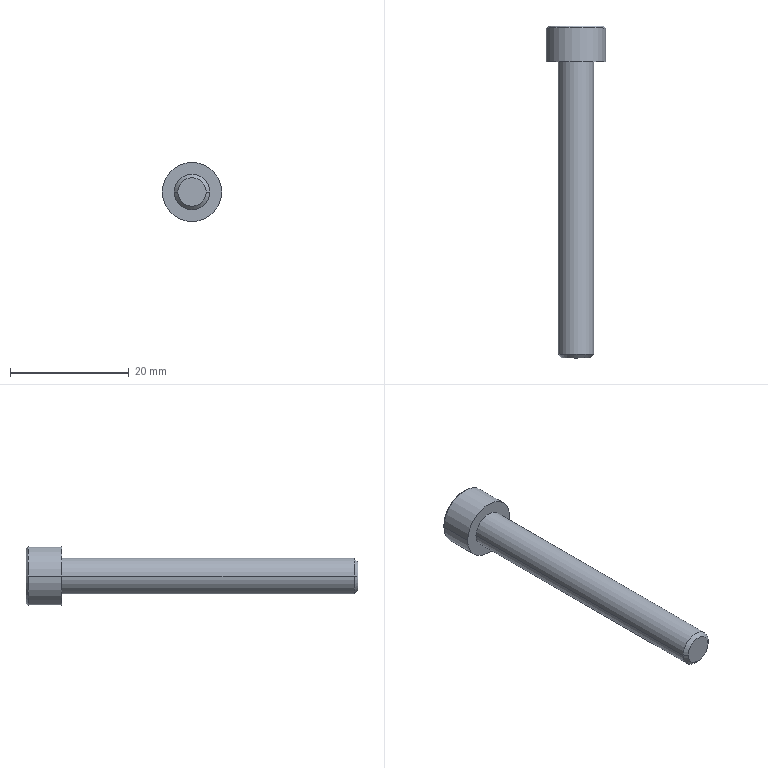Part | SolidWorks | features BaseBody 1, MoveFace 1 | 1 solid | 18 faces | box 10 x 56 x 10 mm | volume 1814 mm3 | plane 10 | cylinder 4 | cone 4 | commonest cylinder face diameters 6 x2 10 x2
STEP:
#1=CARTESIAN_POINT('',(-5.,8.,0.));
#2=VERTEX_POINT('',#1);
#3=CARTESIAN_POINT('',(5.,8.,0.));
#4=VERTEX_POINT('',#3);
#5=CARTESIAN_POINT('',(0.,8.,0.));
#6=DIRECTION('',(0.,1.,0.));
#7=DIRECTION('',(-1.,0.,0.));
#8=AXIS2_PLACEMENT_3D('',#5,#6,#7);
#9=CIRCLE('',#8,5.);
#10=EDGE_CURVE('',#2,#4,#9,.T.);
#11=ORIENTED_EDGE('',*,*,#10,.T.);
#12=CARTESIAN_POINT('',(5.,13.667,0.));
#13=VERTEX_POINT('',#12);
#14=CARTESIAN_POINT('',(5.,0.,0.));
#15=DIRECTION('',(0.,1.,0.));
#16=VECTOR('',#15,1000.);
#17=LINE('',#14,#16);
#18=EDGE_CURVE('',#4,#13,#17,.T.);
#19=ORIENTED_EDGE('',*,*,#18,.T.);
#20=CARTESIAN_POINT('',(-5.,13.667,0.));
#21=VERTEX_POINT('',#20);
#22=CARTESIAN_POINT('',(0.,13.667,0.));
#23=DIRECTION('',(0.,-1.,0.));
#24=DIRECTION('',(-1.,0.,0.));
#25=AXIS2_PLACEMENT_3D('',#22,#23,#24);
#26=CIRCLE('',#25,5.);
#27=EDGE_CURVE('',#13,#21,#26,.T.);
#28=ORIENTED_EDGE('',*,*,#27,.T.);
#29=CARTESIAN_POINT('',(-5.,0.,0.));
#30=DIRECTION('',(0.,1.,0.));
#31=VECTOR('',#30,1000.);
#32=LINE('',#29,#31);
#33=EDGE_CURVE('',#2,#21,#32,.T.);
#34=ORIENTED_EDGE('',*,*,#33,.F.);
#35=EDGE_LOOP('',(#11,#19,#28,#34));
#36=FACE_OUTER_BOUND('',#35,.T.);
#37=CARTESIAN_POINT('',(0.,0.,0.));
#38=DIRECTION('',(0.,1.,0.));
#39=DIRECTION('',(-1.,0.,0.));
#40=AXIS2_PLACEMENT_3D('',#37,#38,#39);
#41=CYLINDRICAL_SURFACE('',#40,5.);
#42=ADVANCED_FACE('',(#36),#41,.T.);
#43=CARTESIAN_POINT('',(4.667,14.,0.));
#44=VERTEX_POINT('',#43);
#45=CARTESIAN_POINT('',(-4.667,14.,0.));
#46=VERTEX_POINT('',#45);
#47=CARTESIAN_POINT('',(0.,14.,0.));
#48=DIRECTION('',(0.,-1.,0.));
#49=DIRECTION('',(1.,0.,0.));
#50=AXIS2_PLACEMENT_3D('',#47,#48,#49);
#51=CIRCLE('',#50,4.667);
#52=EDGE_CURVE('',#44,#46,#51,.T.);
#53=ORIENTED_EDGE('',*,*,#52,.T.);
#54=CARTESIAN_POINT('',(-5.,13.667,0.));
#55=DIRECTION('',(-0.7071,-0.7071,0.));
#56=VECTOR('',#55,1000.);
#57=LINE('',#54,#56);
#58=EDGE_CURVE('',#46,#21,#57,.T.);
#59=ORIENTED_EDGE('',*,*,#58,.T.);
#60=ORIENTED_EDGE('',*,*,#27,.F.);
#61=CARTESIAN_POINT('',(5.,13.667,0.));
#62=DIRECTION('',(0.7071,-0.7071,0.));
#63=VECTOR('',#62,1000.);
#64=LINE('',#61,#63);
#65=EDGE_CURVE('',#44,#13,#64,.T.);
#66=ORIENTED_EDGE('',*,*,#65,.F.);
#67=EDGE_LOOP('',(#53,#59,#60,#66));
#68=FACE_OUTER_BOUND('',#67,.T.);
#69=CARTESIAN_POINT('',(0.,13.667,0.));
#70=DIRECTION('',(0.,-1.,0.));
#71=DIRECTION('',(1.,0.,0.));
#72=AXIS2_PLACEMENT_3D('',#69,#70,#71);
#73=CONICAL_SURFACE('',#72,5.,0.7854);
#74=ADVANCED_FACE('',(#68),#73,.T.);
#75=CARTESIAN_POINT('',(-3.,-41.386,0.));
#76=VERTEX_POINT('',#75);
#77=CARTESIAN_POINT('',(3.,-41.386,0.));
#78=VERTEX_POINT('',#77);
#79=CARTESIAN_POINT('',(0.,-41.386,0.));
#80=DIRECTION('',(0.,1.,0.));
#81=DIRECTION('',(-1.,0.,0.));
#82=AXIS2_PLACEMENT_3D('',#79,#80,#81);
#83=CIRCLE('',#82,3.);
#84=EDGE_CURVE('',#76,#78,#83,.T.);
#85=ORIENTED_EDGE('',*,*,#84,.T.);
#86=CARTESIAN_POINT('',(3.,8.,0.));
#87=VERTEX_POINT('',#86);
#88=CARTESIAN_POINT('',(3.,0.,0.));
#89=DIRECTION('',(0.,1.,0.));
#90=VECTOR('',#89,1000.);
#91=LINE('',#88,#90);
#92=EDGE_CURVE('',#78,#87,#91,.T.);
#93=ORIENTED_EDGE('',*,*,#92,.T.);
#94=CARTESIAN_POINT('',(-3.,8.,0.));
#95=VERTEX_POINT('',#94);
#96=CARTESIAN_POINT('',(0.,8.,0.));
#97=DIRECTION('',(0.,-1.,0.));
#98=DIRECTION('',(-1.,0.,0.));
#99=AXIS2_PLACEMENT_3D('',#96,#97,#98);
#100=CIRCLE('',#99,3.);
#101=EDGE_CURVE('',#87,#95,#100,.T.);
#102=ORIENTED_EDGE('',*,*,#101,.T.);
#103=CARTESIAN_POINT('',(-3.,0.,0.));
#104=DIRECTION('',(0.,1.,0.));
#105=VECTOR('',#104,1000.);
#106=LINE('',#103,#105);
#107=EDGE_CURVE('',#76,#95,#106,.T.);
#108=ORIENTED_EDGE('',*,*,#107,.F.);
#109=EDGE_LOOP('',(#85,#93,#102,#108));
#110=FACE_OUTER_BOUND('',#109,.T.);
#111=CARTESIAN_POINT('',(0.,0.,0.));
#112=DIRECTION('',(0.,1.,0.));
#113=DIRECTION('',(-1.,0.,0.));
#114=AXIS2_PLACEMENT_3D('',#111,#112,#113);
#115=CYLINDRICAL_SURFACE('',#114,3.);
#116=ADVANCED_FACE('',(#110),#115,.T.);
#117=CARTESIAN_POINT('',(-2.386,-42.,0.));
#118=VERTEX_POINT('',#117);
#119=CARTESIAN_POINT('',(2.386,-42.,0.));
#120=VERTEX_POINT('',#119);
#121=CARTESIAN_POINT('',(0.,-42.,0.));
#122=DIRECTION('',(0.,1.,0.));
#123=DIRECTION('',(-1.,0.,0.));
#124=AXIS2_PLACEMENT_3D('',#121,#122,#123);
#125=CIRCLE('',#124,2.386);
#126=EDGE_CURVE('',#118,#120,#125,.T.);
#127=ORIENTED_EDGE('',*,*,#126,.T.);
#128=CARTESIAN_POINT('',(3.,-41.386,0.));
#129=DIRECTION('',(0.7071,0.7071,0.));
#130=VECTOR('',#129,1000.);
#131=LINE('',#128,#130);
#132=EDGE_CURVE('',#120,#78,#131,.T.);
#133=ORIENTED_EDGE('',*,*,#132,.T.);
#134=ORIENTED_EDGE('',*,*,#84,.F.);
#135=CARTESIAN_POINT('',(-3.,-41.386,0.));
#136=DIRECTION('',(-0.7071,0.7071,0.));
#137=VECTOR('',#136,1000.);
#138=LINE('',#135,#137);
#139=EDGE_CURVE('',#118,#76,#138,.T.);
#140=ORIENTED_EDGE('',*,*,#139,.F.);
#141=EDGE_LOOP('',(#127,#133,#134,#140));
#142=FACE_OUTER_BOUND('',#141,.T.);
#143=CARTESIAN_POINT('',(0.,-41.386,0.));
#144=DIRECTION('',(0.,1.,0.));
#145=DIRECTION('',(-1.,0.,0.));
#146=AXIS2_PLACEMENT_3D('',#143,#144,#145);
#147=CONICAL_SURFACE('',#146,3.,0.7854);
#148=ADVANCED_FACE('',(#142),#147,.T.);
#149=ORIENTED_EDGE('',*,*,#18,.F.);
#150=CARTESIAN_POINT('',(0.,8.,0.));
#151=DIRECTION('',(0.,1.,0.));
#152=DIRECTION('',(-1.,0.,0.));
#153=AXIS2_PLACEMENT_3D('',#150,#151,#152);
#154=CIRCLE('',#153,5.);
#155=EDGE_CURVE('',#4,#2,#154,.T.);
#156=ORIENTED_EDGE('',*,*,#155,.T.);
#157=ORIENTED_EDGE('',*,*,#33,.T.);
#158=CARTESIAN_POINT('',(0.,13.667,0.));
#159=DIRECTION('',(0.,-1.,0.));
#160=DIRECTION('',(-1.,0.,0.));
#161=AXIS2_PLACEMENT_3D('',#158,#159,#160);
#162=CIRCLE('',#161,5.);
#163=EDGE_CURVE('',#21,#13,#162,.T.);
#164=ORIENTED_EDGE('',*,*,#163,.T.);
#165=EDGE_LOOP('',(#149,#156,#157,#164));
#166=FACE_OUTER_BOUND('',#165,.T.);
#167=CARTESIAN_POINT('',(0.,0.,0.));
#168=DIRECTION('',(0.,1.,0.));
#169=DIRECTION('',(-1.,0.,0.));
#170=AXIS2_PLACEMENT_3D('',#167,#168,#169);
#171=CYLINDRICAL_SURFACE('',#170,5.);
#172=ADVANCED_FACE('',(#166),#171,.T.);
#173=ORIENTED_EDGE('',*,*,#58,.F.);
#174=CARTESIAN_POINT('',(0.,14.,0.));
#175=DIRECTION('',(0.,-1.,0.));
#176=DIRECTION('',(1.,0.,0.));
#177=AXIS2_PLACEMENT_3D('',#174,#175,#176);
#178=CIRCLE('',#177,4.667);
#179=EDGE_CURVE('',#46,#44,#178,.T.);
#180=ORIENTED_EDGE('',*,*,#179,.T.);
#181=ORIENTED_EDGE('',*,*,#65,.T.);
#182=ORIENTED_EDGE('',*,*,#163,.F.);
#183=EDGE_LOOP('',(#173,#180,#181,#182));
#184=FACE_OUTER_BOUND('',#183,.T.);
#185=CARTESIAN_POINT('',(0.,13.667,0.));
#186=DIRECTION('',(0.,-1.,0.));
#187=DIRECTION('',(1.,0.,0.));
#188=AXIS2_PLACEMENT_3D('',#185,#186,#187);
#189=CONICAL_SURFACE('',#188,5.,0.7854);
#190=ADVANCED_FACE('',(#184),#189,.T.);
#191=ORIENTED_EDGE('',*,*,#10,.F.);
#192=ORIENTED_EDGE('',*,*,#155,.F.);
#193=EDGE_LOOP('',(#191,#192));
#194=FACE_OUTER_BOUND('',#193,.T.);
#195=CARTESIAN_POINT('',(0.,8.,0.));
#196=DIRECTION('',(0.,-1.,0.));
#197=DIRECTION('',(-1.,0.,0.));
#198=AXIS2_PLACEMENT_3D('',#195,#196,#197);
#199=CIRCLE('',#198,3.);
#200=EDGE_CURVE('',#95,#87,#199,.T.);
#201=ORIENTED_EDGE('',*,*,#200,.F.);
#202=ORIENTED_EDGE('',*,*,#101,.F.);
#203=EDGE_LOOP('',(#201,#202));
#204=FACE_BOUND('',#203,.T.);
#205=CARTESIAN_POINT('',(5.,8.,0.));
#206=DIRECTION('',(0.,1.,0.));
#207=DIRECTION('',(-1.,0.,0.));
#208=AXIS2_PLACEMENT_3D('',#205,#206,#207);
#209=PLANE('',#208);
#210=ADVANCED_FACE('',(#194,#204),#209,.F.);
#211=CARTESIAN_POINT('',(-2.51,14.,1.449));
#212=VERTEX_POINT('',#211);
#213=CARTESIAN_POINT('',(0.,14.,2.898));
#214=VERTEX_POINT('',#213);
#215=CARTESIAN_POINT('',(-2.51,14.,1.449));
#216=DIRECTION('',(0.866,0.,0.5));
#217=VECTOR('',#216,1000.);
#218=LINE('',#215,#217);
#219=EDGE_CURVE('',#212,#214,#218,.T.);
#220=ORIENTED_EDGE('',*,*,#219,.F.);
#221=CARTESIAN_POINT('',(-2.51,14.,-1.449));
#222=VERTEX_POINT('',#221);
#223=CARTESIAN_POINT('',(-2.51,14.,0.));
#224=DIRECTION('',(0.,0.,1.));
#225=VECTOR('',#224,1000.);
#226=LINE('',#223,#225);
#227=EDGE_CURVE('',#222,#212,#226,.T.);
#228=ORIENTED_EDGE('',*,*,#227,.F.);
#229=CARTESIAN_POINT('',(0.,14.,-2.898));
#230=VERTEX_POINT('',#229);
#231=CARTESIAN_POINT('',(0.,14.,-2.898));
#232=DIRECTION('',(-0.866,0.,0.5));
#233=VECTOR('',#232,1000.);
#234=LINE('',#231,#233);
#235=EDGE_CURVE('',#230,#222,#234,.T.);
#236=ORIENTED_EDGE('',*,*,#235,.F.);
#237=CARTESIAN_POINT('',(2.51,14.,-1.449));
#238=VERTEX_POINT('',#237);
#239=CARTESIAN_POINT('',(2.51,14.,-1.449));
#240=DIRECTION('',(-0.866,0.,-0.5));
#241=VECTOR('',#240,1000.);
#242=LINE('',#239,#241);
#243=EDGE_CURVE('',#238,#230,#242,.T.);
#244=ORIENTED_EDGE('',*,*,#243,.F.);
#245=CARTESIAN_POINT('',(2.51,14.,1.449));
#246=VERTEX_POINT('',#245);
#247=CARTESIAN_POINT('',(2.51,14.,0.));
#248=DIRECTION('',(0.,0.,-1.));
#249=VECTOR('',#248,1000.);
#250=LINE('',#247,#249);
#251=EDGE_CURVE('',#246,#238,#250,.T.);
#252=ORIENTED_EDGE('',*,*,#251,.F.);
#253=CARTESIAN_POINT('',(0.,14.,2.898));
#254=DIRECTION('',(0.866,0.,-0.5));
#255=VECTOR('',#254,1000.);
#256=LINE('',#253,#255);
#257=EDGE_CURVE('',#214,#246,#256,.T.);
#258=ORIENTED_EDGE('',*,*,#257,.F.);
#259=EDGE_LOOP('',(#220,#228,#236,#244,#252,#258));
#260=FACE_BOUND('',#259,.T.);
#261=ORIENTED_EDGE('',*,*,#52,.F.);
#262=ORIENTED_EDGE('',*,*,#179,.F.);
#263=EDGE_LOOP('',(#261,#262));
#264=FACE_OUTER_BOUND('',#263,.T.);
#265=CARTESIAN_POINT('',(0.,14.,0.));
#266=DIRECTION('',(0.,-1.,0.));
#267=DIRECTION('',(1.,0.,0.));
#268=AXIS2_PLACEMENT_3D('',#265,#266,#267);
#269=PLANE('',#268);
#270=ADVANCED_FACE('',(#260,#264),#269,.F.);
#271=ORIENTED_EDGE('',*,*,#92,.F.);
#272=CARTESIAN_POINT('',(0.,-41.386,0.));
#273=DIRECTION('',(0.,1.,0.));
#274=DIRECTION('',(-1.,0.,0.));
#275=AXIS2_PLACEMENT_3D('',#272,#273,#274);
#276=CIRCLE('',#275,3.);
#277=EDGE_CURVE('',#78,#76,#276,.T.);
#278=ORIENTED_EDGE('',*,*,#277,.T.);
#279=ORIENTED_EDGE('',*,*,#107,.T.);
#280=ORIENTED_EDGE('',*,*,#200,.T.);
#281=EDGE_LOOP('',(#271,#278,#279,#280));
#282=FACE_OUTER_BOUND('',#281,.T.);
#283=CARTESIAN_POINT('',(0.,0.,0.));
#284=DIRECTION('',(0.,1.,0.));
#285=DIRECTION('',(-1.,0.,0.));
#286=AXIS2_PLACEMENT_3D('',#283,#284,#285);
#287=CYLINDRICAL_SURFACE('',#286,3.);
#288=ADVANCED_FACE('',(#282),#287,.T.);
#289=CARTESIAN_POINT('',(2.51,11.,1.449));
#290=VERTEX_POINT('',#289);
#291=CARTESIAN_POINT('',(2.51,11.,1.449));
#292=DIRECTION('',(0.,1.,0.));
#293=VECTOR('',#292,1000.);
#294=LINE('',#291,#293);
#295=EDGE_CURVE('',#290,#246,#294,.T.);
#296=ORIENTED_EDGE('',*,*,#295,.F.);
#297=CARTESIAN_POINT('',(0.,11.,2.898));
#298=VERTEX_POINT('',#297);
#299=CARTESIAN_POINT('',(0.,11.,2.898));
#300=DIRECTION('',(0.866,0.,-0.5));
#301=VECTOR('',#300,1000.);
#302=LINE('',#299,#301);
#303=EDGE_CURVE('',#298,#290,#302,.T.);
#304=ORIENTED_EDGE('',*,*,#303,.F.);
#305=CARTESIAN_POINT('',(0.,11.,2.898));
#306=DIRECTION('',(0.,-1.,0.));
#307=VECTOR('',#306,1000.);
#308=LINE('',#305,#307);
#309=EDGE_CURVE('',#214,#298,#308,.T.);
#310=ORIENTED_EDGE('',*,*,#309,.F.);
#311=ORIENTED_EDGE('',*,*,#257,.T.);
#312=EDGE_LOOP('',(#296,#304,#310,#311));
#313=FACE_OUTER_BOUND('',#312,.T.);
#314=CARTESIAN_POINT('',(0.,11.,2.898));
#315=DIRECTION('',(0.5,0.,0.866));
#316=DIRECTION('',(0.866,0.,-0.5));
#317=AXIS2_PLACEMENT_3D('',#314,#315,#316);
#318=PLANE('',#317);
#319=ADVANCED_FACE('',(#313),#318,.F.);
#320=ORIENTED_EDGE('',*,*,#309,.T.);
#321=CARTESIAN_POINT('',(-2.51,11.,1.449));
#322=VERTEX_POINT('',#321);
#323=CARTESIAN_POINT('',(-2.51,11.,1.449));
#324=DIRECTION('',(0.866,0.,0.5));
#325=VECTOR('',#324,1000.);
#326=LINE('',#323,#325);
#327=EDGE_CURVE('',#322,#298,#326,.T.);
#328=ORIENTED_EDGE('',*,*,#327,.F.);
#329=CARTESIAN_POINT('',(-2.51,11.,1.449));
#330=DIRECTION('',(0.,-1.,0.));
#331=VECTOR('',#330,1000.);
#332=LINE('',#329,#331);
#333=EDGE_CURVE('',#212,#322,#332,.T.);
#334=ORIENTED_EDGE('',*,*,#333,.F.);
#335=ORIENTED_EDGE('',*,*,#219,.T.);
#336=EDGE_LOOP('',(#320,#328,#334,#335));
#337=FACE_OUTER_BOUND('',#336,.T.);
#338=CARTESIAN_POINT('',(-2.51,11.,1.449));
#339=DIRECTION('',(-0.5,0.,0.866));
#340=DIRECTION('',(0.866,0.,0.5));
#341=AXIS2_PLACEMENT_3D('',#338,#339,#340);
#342=PLANE('',#341);
#343=ADVANCED_FACE('',(#337),#342,.F.);
#344=ORIENTED_EDGE('',*,*,#333,.T.);
#345=CARTESIAN_POINT('',(-2.51,11.,-1.449));
#346=VERTEX_POINT('',#345);
#347=CARTESIAN_POINT('',(-2.51,11.,-1.449));
#348=DIRECTION('',(0.,0.,1.));
#349=VECTOR('',#348,1000.);
#350=LINE('',#347,#349);
#351=EDGE_CURVE('',#346,#322,#350,.T.);
#352=ORIENTED_EDGE('',*,*,#351,.F.);
#353=CARTESIAN_POINT('',(-2.51,11.,-1.449));
#354=DIRECTION('',(0.,-1.,0.));
#355=VECTOR('',#354,1000.);
#356=LINE('',#353,#355);
#357=EDGE_CURVE('',#222,#346,#356,.T.);
#358=ORIENTED_EDGE('',*,*,#357,.F.);
#359=ORIENTED_EDGE('',*,*,#227,.T.);
#360=EDGE_LOOP('',(#344,#352,#358,#359));
#361=FACE_OUTER_BOUND('',#360,.T.);
#362=CARTESIAN_POINT('',(-2.51,11.,-1.449));
#363=DIRECTION('',(-1.,0.,0.));
#364=DIRECTION('',(0.,0.,1.));
#365=AXIS2_PLACEMENT_3D('',#362,#363,#364);
#366=PLANE('',#365);
#367=ADVANCED_FACE('',(#361),#366,.F.);
#368=ORIENTED_EDGE('',*,*,#357,.T.);
#369=CARTESIAN_POINT('',(0.,11.,-2.898));
#370=VERTEX_POINT('',#369);
#371=CARTESIAN_POINT('',(0.,11.,-2.898));
#372=DIRECTION('',(-0.866,0.,0.5));
#373=VECTOR('',#372,1000.);
#374=LINE('',#371,#373);
#375=EDGE_CURVE('',#370,#346,#374,.T.);
#376=ORIENTED_EDGE('',*,*,#375,.F.);
#377=CARTESIAN_POINT('',(0.,11.,-2.898));
#378=DIRECTION('',(0.,-1.,0.));
#379=VECTOR('',#378,1000.);
#380=LINE('',#377,#379);
#381=EDGE_CURVE('',#230,#370,#380,.T.);
#382=ORIENTED_EDGE('',*,*,#381,.F.);
#383=ORIENTED_EDGE('',*,*,#235,.T.);
#384=EDGE_LOOP('',(#368,#376,#382,#383));
#385=FACE_OUTER_BOUND('',#384,.T.);
#386=CARTESIAN_POINT('',(0.,11.,-2.898));
#387=DIRECTION('',(-0.5,0.,-0.866));
#388=DIRECTION('',(-0.866,0.,0.5));
#389=AXIS2_PLACEMENT_3D('',#386,#387,#388);
#390=PLANE('',#389);
#391=ADVANCED_FACE('',(#385),#390,.F.);
#392=ORIENTED_EDGE('',*,*,#381,.T.);
#393=CARTESIAN_POINT('',(2.51,11.,-1.449));
#394=VERTEX_POINT('',#393);
#395=CARTESIAN_POINT('',(2.51,11.,-1.449));
#396=DIRECTION('',(-0.866,0.,-0.5));
#397=VECTOR('',#396,1000.);
#398=LINE('',#395,#397);
#399=EDGE_CURVE('',#394,#370,#398,.T.);
#400=ORIENTED_EDGE('',*,*,#399,.F.);
#401=CARTESIAN_POINT('',(2.51,11.,-1.449));
#402=DIRECTION('',(0.,-1.,0.));
#403=VECTOR('',#402,1000.);
#404=LINE('',#401,#403);
#405=EDGE_CURVE('',#238,#394,#404,.T.);
#406=ORIENTED_EDGE('',*,*,#405,.F.);
#407=ORIENTED_EDGE('',*,*,#243,.T.);
#408=EDGE_LOOP('',(#392,#400,#406,#407));
#409=FACE_OUTER_BOUND('',#408,.T.);
#410=CARTESIAN_POINT('',(2.51,11.,-1.449));
#411=DIRECTION('',(0.5,0.,-0.866));
#412=DIRECTION('',(-0.866,0.,-0.5));
#413=AXIS2_PLACEMENT_3D('',#410,#411,#412);
#414=PLANE('',#413);
#415=ADVANCED_FACE('',(#409),#414,.F.);
#416=ORIENTED_EDGE('',*,*,#251,.T.);
#417=ORIENTED_EDGE('',*,*,#405,.T.);
#418=CARTESIAN_POINT('',(2.51,11.,1.449));
#419=DIRECTION('',(0.,0.,-1.));
#420=VECTOR('',#419,1000.);
#421=LINE('',#418,#420);
#422=EDGE_CURVE('',#290,#394,#421,.T.);
#423=ORIENTED_EDGE('',*,*,#422,.F.);
#424=ORIENTED_EDGE('',*,*,#295,.T.);
#425=EDGE_LOOP('',(#416,#417,#423,#424));
#426=FACE_OUTER_BOUND('',#425,.T.);
#427=CARTESIAN_POINT('',(2.51,11.,1.449));
#428=DIRECTION('',(1.,0.,0.));
#429=DIRECTION('',(0.,0.,-1.));
#430=AXIS2_PLACEMENT_3D('',#427,#428,#429);
#431=PLANE('',#430);
#432=ADVANCED_FACE('',(#426),#431,.F.);
#433=ORIENTED_EDGE('',*,*,#132,.F.);
#434=CARTESIAN_POINT('',(0.,-42.,0.));
#435=DIRECTION('',(0.,1.,0.));
#436=DIRECTION('',(-1.,0.,0.));
#437=AXIS2_PLACEMENT_3D('',#434,#435,#436);
#438=CIRCLE('',#437,2.386);
#439=EDGE_CURVE('',#120,#118,#438,.T.);
#440=ORIENTED_EDGE('',*,*,#439,.T.);
#441=ORIENTED_EDGE('',*,*,#139,.T.);
#442=ORIENTED_EDGE('',*,*,#277,.F.);
#443=EDGE_LOOP('',(#433,#440,#441,#442));
#444=FACE_OUTER_BOUND('',#443,.T.);
#445=CARTESIAN_POINT('',(0.,-41.386,0.));
#446=DIRECTION('',(0.,1.,0.));
#447=DIRECTION('',(-1.,0.,0.));
#448=AXIS2_PLACEMENT_3D('',#445,#446,#447);
#449=CONICAL_SURFACE('',#448,3.,0.7854);
#450=ADVANCED_FACE('',(#444),#449,.T.);
#451=ORIENTED_EDGE('',*,*,#399,.T.);
#452=ORIENTED_EDGE('',*,*,#375,.T.);
#453=ORIENTED_EDGE('',*,*,#351,.T.);
#454=ORIENTED_EDGE('',*,*,#327,.T.);
#455=ORIENTED_EDGE('',*,*,#303,.T.);
#456=ORIENTED_EDGE('',*,*,#422,.T.);
#457=EDGE_LOOP('',(#451,#452,#453,#454,#455,#456));
#458=FACE_OUTER_BOUND('',#457,.T.);
#459=CARTESIAN_POINT('',(0.,11.,0.));
#460=DIRECTION('',(0.,1.,0.));
#461=DIRECTION('',(0.,0.,1.));
#462=AXIS2_PLACEMENT_3D('',#459,#460,#461);
#463=PLANE('',#462);
#464=ADVANCED_FACE('',(#458),#463,.T.);
#465=ORIENTED_EDGE('',*,*,#126,.F.);
#466=ORIENTED_EDGE('',*,*,#439,.F.);
#467=EDGE_LOOP('',(#465,#466));
#468=FACE_OUTER_BOUND('',#467,.T.);
#469=CARTESIAN_POINT('',(2.386,-42.,0.));
#470=DIRECTION('',(0.,1.,0.));
#471=DIRECTION('',(-1.,0.,0.));
#472=AXIS2_PLACEMENT_3D('',#469,#470,#471);
#473=PLANE('',#472);
#474=ADVANCED_FACE('',(#468),#473,.F.);
#475=CLOSED_SHELL('',(#42,#74,#116,#148,#172,#190,#210,#270,#288,#319,#343,#367,#391,#415,#432,#450,#464,#474));
#476=MANIFOLD_SOLID_BREP('',#475);
#477=CARTESIAN_POINT('',(0.,0.,0.));
#478=DIRECTION('',(0.,0.,1.));
#479=DIRECTION('',(1.,0.,0.));
#480=AXIS2_PLACEMENT_3D('',#477,#478,#479);
#481=(LENGTH_UNIT()NAMED_UNIT(*)SI_UNIT(.MILLI.,.METRE.));
#482=UNCERTAINTY_MEASURE_WITH_UNIT(LENGTH_MEASURE(0.00001),#481,'','');
#483=(NAMED_UNIT(*)PLANE_ANGLE_UNIT()SI_UNIT($,.RADIAN.));
#484=(NAMED_UNIT(*)SI_UNIT($,.STERADIAN.)SOLID_ANGLE_UNIT());
#485=(GEOMETRIC_REPRESENTATION_CONTEXT(3)GLOBAL_UNCERTAINTY_ASSIGNED_CONTEXT((#482))GLOBAL_UNIT_ASSIGNED_CONTEXT((#481,#483,#484))REPRESENTATION_CONTEXT('',''));
#486=ADVANCED_BREP_SHAPE_REPRESENTATION('',(#476,#480),#485);